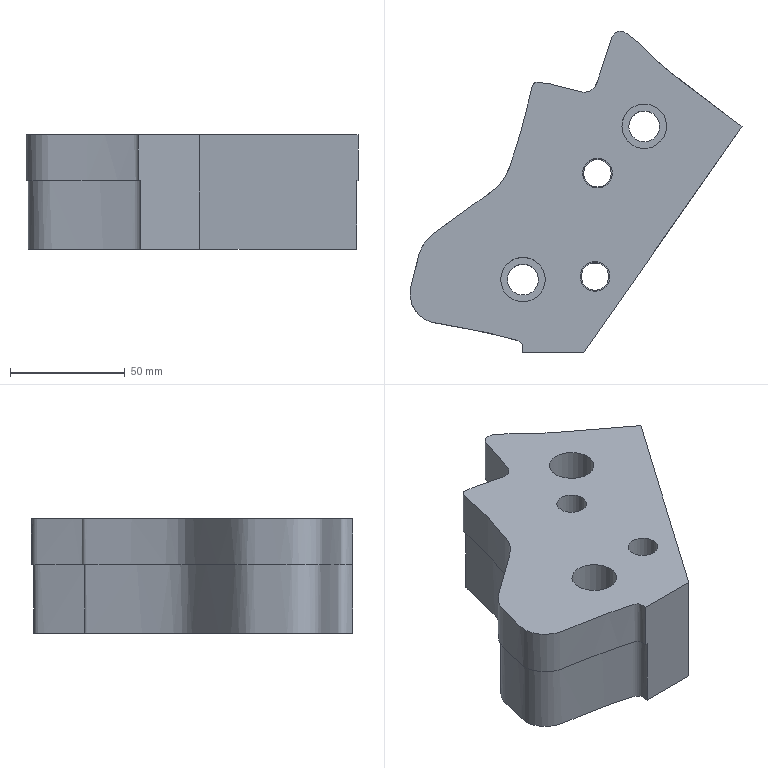Part | NX | features solid 2 | 1 solid | 19 faces | box 144.972 x 140.193 x 50 mm | volume 503564 mm3 | plane 9 | cylinder 8 | spline 2 | commonest cylinder face diameters 12 x2 13 x2 13.5 x2 19.5 x2